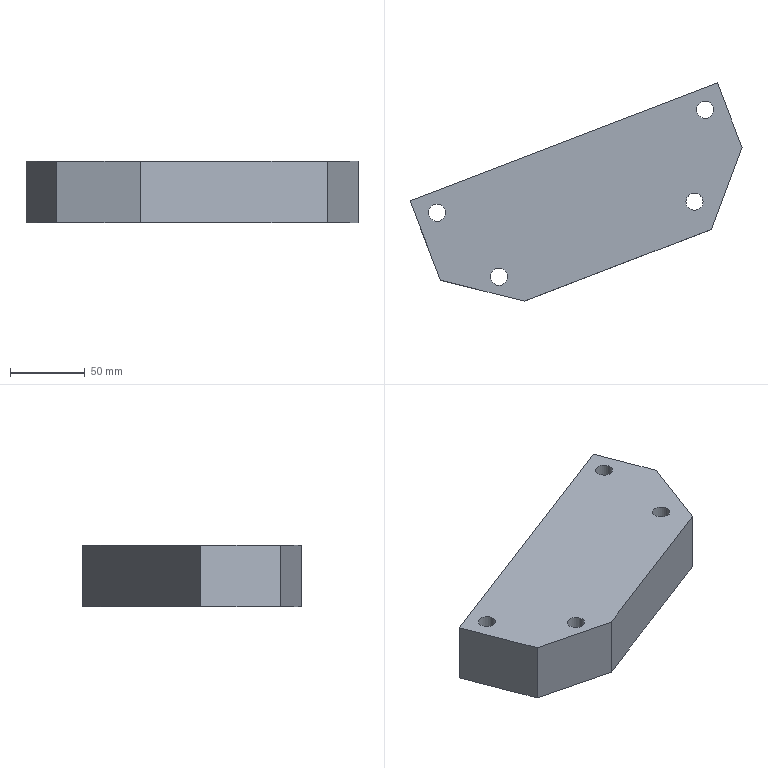Part | NX | features solid 2 | 1 solid | 20 faces | box 221.896 x 145.899 x 41 mm | volume 719760 mm3 | plane 12 | cylinder 8 | commonest cylinder face diameters 11.5 x4 18 x4
STEP:
#1=CARTESIAN_POINT('',(970.121,174.216,73.));
#2=VERTEX_POINT('',#1);
#3=CARTESIAN_POINT('',(968.06,179.584,73.));
#4=DIRECTION('',(0.,0.,-1.));
#5=DIRECTION('',(0.3584,-0.9336,0.));
#6=AXIS2_PLACEMENT_3D('',#3,#4,#5);
#7=CIRCLE('',#6,5.75);
#8=EDGE_CURVE('',#2,#2,#7,.T.);
#9=ORIENTED_EDGE('',*,*,#8,.F.);
#10=EDGE_LOOP('',(#9));
#11=FACE_BOUND('',#10,.T.);
#12=CARTESIAN_POINT('',(971.285,171.182,73.));
#13=VERTEX_POINT('',#12);
#14=CARTESIAN_POINT('',(968.06,179.584,73.));
#15=DIRECTION('',(0.,0.,-1.));
#16=DIRECTION('',(0.3584,-0.9336,0.));
#17=AXIS2_PLACEMENT_3D('',#14,#15,#16);
#18=CIRCLE('',#17,9.);
#19=EDGE_CURVE('',#13,#13,#18,.T.);
#20=ORIENTED_EDGE('',*,*,#19,.T.);
#21=EDGE_LOOP('',(#20));
#22=FACE_BOUND('',#21,.T.);
#23=CARTESIAN_POINT('',(968.06,179.584,73.));
#24=DIRECTION('',(0.,0.,1.));
#25=DIRECTION('',(-0.3584,0.9336,0.));
#26=AXIS2_PLACEMENT_3D('',#23,#24,#25);
#27=PLANE('',#26);
#28=ADVANCED_FACE('',(#11,#22),#27,.F.);
#29=CARTESIAN_POINT('',(1011.473,131.478,73.));
#30=VERTEX_POINT('',#29);
#31=CARTESIAN_POINT('',(1009.413,136.846,73.));
#32=DIRECTION('',(0.,0.,-1.));
#33=DIRECTION('',(0.3584,-0.9336,0.));
#34=AXIS2_PLACEMENT_3D('',#31,#32,#33);
#35=CIRCLE('',#34,5.75);
#36=EDGE_CURVE('',#30,#30,#35,.T.);
#37=ORIENTED_EDGE('',*,*,#36,.F.);
#38=EDGE_LOOP('',(#37));
#39=FACE_BOUND('',#38,.T.);
#40=CARTESIAN_POINT('',(1012.638,128.444,73.));
#41=VERTEX_POINT('',#40);
#42=CARTESIAN_POINT('',(1009.413,136.846,73.));
#43=DIRECTION('',(0.,0.,-1.));
#44=DIRECTION('',(0.3584,-0.9336,0.));
#45=AXIS2_PLACEMENT_3D('',#42,#43,#44);
#46=CIRCLE('',#45,9.);
#47=EDGE_CURVE('',#41,#41,#46,.T.);
#48=ORIENTED_EDGE('',*,*,#47,.T.);
#49=EDGE_LOOP('',(#48));
#50=FACE_BOUND('',#49,.T.);
#51=CARTESIAN_POINT('',(1009.413,136.846,73.));
#52=DIRECTION('',(0.,0.,1.));
#53=DIRECTION('',(-0.3584,0.9336,0.));
#54=AXIS2_PLACEMENT_3D('',#51,#52,#53);
#55=PLANE('',#54);
#56=ADVANCED_FACE('',(#39,#50),#55,.F.);
#57=CARTESIAN_POINT('',(1149.368,243.023,73.));
#58=VERTEX_POINT('',#57);
#59=CARTESIAN_POINT('',(1147.307,248.391,73.));
#60=DIRECTION('',(0.,0.,-1.));
#61=DIRECTION('',(0.3584,-0.9336,0.));
#62=AXIS2_PLACEMENT_3D('',#59,#60,#61);
#63=CIRCLE('',#62,5.75);
#64=EDGE_CURVE('',#58,#58,#63,.T.);
#65=ORIENTED_EDGE('',*,*,#64,.F.);
#66=EDGE_LOOP('',(#65));
#67=FACE_BOUND('',#66,.T.);
#68=CARTESIAN_POINT('',(1150.533,239.989,73.));
#69=VERTEX_POINT('',#68);
#70=CARTESIAN_POINT('',(1147.307,248.391,73.));
#71=DIRECTION('',(0.,0.,-1.));
#72=DIRECTION('',(0.3584,-0.9336,0.));
#73=AXIS2_PLACEMENT_3D('',#70,#71,#72);
#74=CIRCLE('',#73,9.);
#75=EDGE_CURVE('',#69,#69,#74,.T.);
#76=ORIENTED_EDGE('',*,*,#75,.T.);
#77=EDGE_LOOP('',(#76));
#78=FACE_BOUND('',#77,.T.);
#79=CARTESIAN_POINT('',(1044.614,208.97,73.));
#80=DIRECTION('',(0.,0.,1.));
#81=DIRECTION('',(-0.3584,0.9336,0.));
#82=AXIS2_PLACEMENT_3D('',#79,#80,#81);
#83=PLANE('',#82);
#84=ADVANCED_FACE('',(#67,#78),#83,.F.);
#85=CARTESIAN_POINT('',(1026.418,120.579,60.));
#86=VERTEX_POINT('',#85);
#87=CARTESIAN_POINT('',(1026.418,120.579,101.));
#88=VERTEX_POINT('',#87);
#89=CARTESIAN_POINT('',(1026.418,120.579,-25.));
#90=DIRECTION('',(0.,0.,1.));
#91=VECTOR('',#90,1000.);
#92=LINE('',#89,#91);
#93=EDGE_CURVE('',#86,#88,#92,.T.);
#94=ORIENTED_EDGE('',*,*,#93,.T.);
#95=CARTESIAN_POINT('',(970.348,134.558,101.));
#96=VERTEX_POINT('',#95);
#97=CARTESIAN_POINT('',(1046.37,115.604,101.));
#98=DIRECTION('',(-0.9703,0.2419,0.));
#99=VECTOR('',#98,1000.);
#100=LINE('',#97,#99);
#101=EDGE_CURVE('',#88,#96,#100,.T.);
#102=ORIENTED_EDGE('',*,*,#101,.T.);
#103=CARTESIAN_POINT('',(970.348,134.558,60.));
#104=VERTEX_POINT('',#103);
#105=CARTESIAN_POINT('',(970.348,134.558,-25.));
#106=DIRECTION('',(0.,0.,-1.));
#107=VECTOR('',#106,1000.);
#108=LINE('',#105,#107);
#109=EDGE_CURVE('',#96,#104,#108,.T.);
#110=ORIENTED_EDGE('',*,*,#109,.T.);
#111=CARTESIAN_POINT('',(1046.37,115.604,60.));
#112=DIRECTION('',(0.9703,-0.2419,0.));
#113=VECTOR('',#112,1000.);
#114=LINE('',#111,#113);
#115=EDGE_CURVE('',#104,#86,#114,.T.);
#116=ORIENTED_EDGE('',*,*,#115,.T.);
#117=EDGE_LOOP('',(#94,#102,#110,#116));
#118=FACE_BOUND('',#117,.T.);
#119=CARTESIAN_POINT('',(1046.37,115.604,-25.));
#120=DIRECTION('',(0.2419,0.9703,0.));
#121=DIRECTION('',(0.,0.,1.));
#122=AXIS2_PLACEMENT_3D('',#119,#120,#121);
#123=PLANE('',#122);
#124=ADVANCED_FACE('',(#118),#123,.F.);
#125=CARTESIAN_POINT('',(949.973,187.637,101.));
#126=VERTEX_POINT('',#125);
#127=CARTESIAN_POINT('',(966.099,145.626,101.));
#128=DIRECTION('',(0.3584,-0.9336,0.));
#129=VECTOR('',#128,1000.);
#130=LINE('',#127,#129);
#131=EDGE_CURVE('',#126,#96,#130,.T.);
#132=ORIENTED_EDGE('',*,*,#131,.F.);
#133=CARTESIAN_POINT('',(949.973,187.637,60.));
#134=VERTEX_POINT('',#133);
#135=CARTESIAN_POINT('',(949.973,187.637,-25.));
#136=DIRECTION('',(0.,0.,1.));
#137=VECTOR('',#136,1000.);
#138=LINE('',#135,#137);
#139=EDGE_CURVE('',#134,#126,#138,.T.);
#140=ORIENTED_EDGE('',*,*,#139,.F.);
#141=CARTESIAN_POINT('',(966.099,145.626,60.));
#142=DIRECTION('',(-0.3584,0.9336,0.));
#143=VECTOR('',#142,1000.);
#144=LINE('',#141,#143);
#145=EDGE_CURVE('',#104,#134,#144,.T.);
#146=ORIENTED_EDGE('',*,*,#145,.F.);
#147=ORIENTED_EDGE('',*,*,#109,.F.);
#148=EDGE_LOOP('',(#132,#140,#146,#147));
#149=FACE_BOUND('',#148,.T.);
#150=CARTESIAN_POINT('',(966.099,145.626,-25.));
#151=DIRECTION('',(-0.9336,-0.3584,0.));
#152=DIRECTION('',(0.,0.,-1.));
#153=AXIS2_PLACEMENT_3D('',#150,#151,#152);
#154=PLANE('',#153);
#155=ADVANCED_FACE('',(#149),#154,.T.);
#156=CARTESIAN_POINT('',(1155.36,266.478,60.));
#157=VERTEX_POINT('',#156);
#158=CARTESIAN_POINT('',(1155.36,266.478,101.));
#159=VERTEX_POINT('',#158);
#160=CARTESIAN_POINT('',(1155.36,266.478,-25.));
#161=DIRECTION('',(0.,0.,1.));
#162=VECTOR('',#161,1000.);
#163=LINE('',#160,#162);
#164=EDGE_CURVE('',#157,#159,#163,.T.);
#165=ORIENTED_EDGE('',*,*,#164,.F.);
#166=CARTESIAN_POINT('',(1001.32,207.347,60.));
#167=DIRECTION('',(0.9336,0.3584,0.));
#168=VECTOR('',#167,1000.);
#169=LINE('',#166,#168);
#170=EDGE_CURVE('',#134,#157,#169,.T.);
#171=ORIENTED_EDGE('',*,*,#170,.F.);
#172=ORIENTED_EDGE('',*,*,#139,.T.);
#173=CARTESIAN_POINT('',(1001.32,207.347,101.));
#174=DIRECTION('',(-0.9336,-0.3584,0.));
#175=VECTOR('',#174,1000.);
#176=LINE('',#173,#175);
#177=EDGE_CURVE('',#159,#126,#176,.T.);
#178=ORIENTED_EDGE('',*,*,#177,.F.);
#179=EDGE_LOOP('',(#165,#171,#172,#178));
#180=FACE_BOUND('',#179,.T.);
#181=CARTESIAN_POINT('',(1001.32,207.347,-25.));
#182=DIRECTION('',(-0.3584,0.9336,0.));
#183=DIRECTION('',(0.,0.,-1.));
#184=AXIS2_PLACEMENT_3D('',#181,#182,#183);
#185=PLANE('',#184);
#186=ADVANCED_FACE('',(#180),#185,.T.);
#187=CARTESIAN_POINT('',(1171.868,223.474,101.));
#188=VERTEX_POINT('',#187);
#189=CARTESIAN_POINT('',(1171.487,224.467,101.));
#190=DIRECTION('',(-0.3584,0.9336,0.));
#191=VECTOR('',#190,1000.);
#192=LINE('',#189,#191);
#193=EDGE_CURVE('',#188,#159,#192,.T.);
#194=ORIENTED_EDGE('',*,*,#193,.F.);
#195=CARTESIAN_POINT('',(1171.868,223.474,60.));
#196=VERTEX_POINT('',#195);
#197=CARTESIAN_POINT('',(1171.868,223.474,-25.));
#198=DIRECTION('',(0.,0.,-1.));
#199=VECTOR('',#198,1000.);
#200=LINE('',#197,#199);
#201=EDGE_CURVE('',#188,#196,#200,.T.);
#202=ORIENTED_EDGE('',*,*,#201,.T.);
#203=CARTESIAN_POINT('',(1171.487,224.467,60.));
#204=DIRECTION('',(0.3584,-0.9336,0.));
#205=VECTOR('',#204,1000.);
#206=LINE('',#203,#205);
#207=EDGE_CURVE('',#157,#196,#206,.T.);
#208=ORIENTED_EDGE('',*,*,#207,.F.);
#209=ORIENTED_EDGE('',*,*,#164,.T.);
#210=EDGE_LOOP('',(#194,#202,#208,#209));
#211=FACE_BOUND('',#210,.T.);
#212=CARTESIAN_POINT('',(1171.487,224.467,-25.));
#213=DIRECTION('',(0.9336,0.3584,0.));
#214=DIRECTION('',(0.,0.,1.));
#215=AXIS2_PLACEMENT_3D('',#212,#213,#214);
#216=PLANE('',#215);
#217=ADVANCED_FACE('',(#211),#216,.T.);
#218=CARTESIAN_POINT('',(1151.325,168.526,60.));
#219=VERTEX_POINT('',#218);
#220=CARTESIAN_POINT('',(1151.325,168.526,101.));
#221=VERTEX_POINT('',#220);
#222=CARTESIAN_POINT('',(1151.325,168.526,-25.));
#223=DIRECTION('',(0.,0.,1.));
#224=VECTOR('',#223,1000.);
#225=LINE('',#222,#224);
#226=EDGE_CURVE('',#219,#221,#225,.T.);
#227=ORIENTED_EDGE('',*,*,#226,.F.);
#228=CARTESIAN_POINT('',(746.976,-912.968,60.));
#229=DIRECTION('',(-0.3502,-0.9367,0.));
#230=VECTOR('',#229,1000.);
#231=LINE('',#228,#230);
#232=EDGE_CURVE('',#196,#219,#231,.T.);
#233=ORIENTED_EDGE('',*,*,#232,.F.);
#234=ORIENTED_EDGE('',*,*,#201,.F.);
#235=CARTESIAN_POINT('',(1234.634,391.351,101.));
#236=DIRECTION('',(0.3502,0.9367,0.));
#237=VECTOR('',#236,1000.);
#238=LINE('',#235,#237);
#239=EDGE_CURVE('',#221,#188,#238,.T.);
#240=ORIENTED_EDGE('',*,*,#239,.F.);
#241=EDGE_LOOP('',(#227,#233,#234,#240));
#242=FACE_BOUND('',#241,.T.);
#243=CARTESIAN_POINT('',(1145.984,154.243,93.));
#244=DIRECTION('',(0.9367,-0.3502,0.));
#245=DIRECTION('',(-0.3502,-0.9367,0.));
#246=AXIS2_PLACEMENT_3D('',#243,#244,#245);
#247=PLANE('',#246);
#248=ADVANCED_FACE('',(#242),#247,.T.);
#249=CARTESIAN_POINT('',(1033.573,123.325,60.));
#250=DIRECTION('',(-0.9336,-0.3584,0.));
#251=VECTOR('',#250,1000.);
#252=LINE('',#249,#251);
#253=EDGE_CURVE('',#219,#86,#252,.T.);
#254=ORIENTED_EDGE('',*,*,#253,.F.);
#255=ORIENTED_EDGE('',*,*,#226,.T.);
#256=CARTESIAN_POINT('',(1033.573,123.325,101.));
#257=DIRECTION('',(0.9336,0.3584,0.));
#258=VECTOR('',#257,1000.);
#259=LINE('',#256,#258);
#260=EDGE_CURVE('',#88,#221,#259,.T.);
#261=ORIENTED_EDGE('',*,*,#260,.F.);
#262=ORIENTED_EDGE('',*,*,#93,.F.);
#263=EDGE_LOOP('',(#254,#255,#261,#262));
#264=FACE_BOUND('',#263,.T.);
#265=CARTESIAN_POINT('',(1033.573,123.325,-25.));
#266=DIRECTION('',(0.3584,-0.9336,0.));
#267=DIRECTION('',(0.,0.,1.));
#268=AXIS2_PLACEMENT_3D('',#265,#266,#267);
#269=PLANE('',#268);
#270=ADVANCED_FACE('',(#264),#269,.T.);
#271=CARTESIAN_POINT('',(970.121,174.216,101.));
#272=VERTEX_POINT('',#271);
#273=CARTESIAN_POINT('',(968.06,179.584,101.));
#274=DIRECTION('',(0.,0.,-1.));
#275=DIRECTION('',(0.3584,-0.9336,0.));
#276=AXIS2_PLACEMENT_3D('',#273,#274,#275);
#277=CIRCLE('',#276,5.75);
#278=EDGE_CURVE('',#272,#272,#277,.T.);
#279=ORIENTED_EDGE('',*,*,#278,.F.);
#280=EDGE_LOOP('',(#279));
#281=FACE_BOUND('',#280,.T.);
#282=ORIENTED_EDGE('',*,*,#8,.T.);
#283=EDGE_LOOP('',(#282));
#284=FACE_BOUND('',#283,.T.);
#285=CARTESIAN_POINT('',(968.06,179.584,55.));
#286=DIRECTION('',(0.,0.,1.));
#287=DIRECTION('',(-0.3584,0.9336,0.));
#288=AXIS2_PLACEMENT_3D('',#285,#286,#287);
#289=CYLINDRICAL_SURFACE('',#288,5.75);
#290=ADVANCED_FACE('',(#281,#284),#289,.F.);
#291=CARTESIAN_POINT('',(1011.473,131.478,101.));
#292=VERTEX_POINT('',#291);
#293=CARTESIAN_POINT('',(1009.413,136.846,101.));
#294=DIRECTION('',(0.,0.,-1.));
#295=DIRECTION('',(0.3584,-0.9336,0.));
#296=AXIS2_PLACEMENT_3D('',#293,#294,#295);
#297=CIRCLE('',#296,5.75);
#298=EDGE_CURVE('',#292,#292,#297,.T.);
#299=ORIENTED_EDGE('',*,*,#298,.F.);
#300=EDGE_LOOP('',(#299));
#301=FACE_BOUND('',#300,.T.);
#302=ORIENTED_EDGE('',*,*,#36,.T.);
#303=EDGE_LOOP('',(#302));
#304=FACE_BOUND('',#303,.T.);
#305=CARTESIAN_POINT('',(1009.413,136.846,55.));
#306=DIRECTION('',(0.,0.,1.));
#307=DIRECTION('',(-0.3584,0.9336,0.));
#308=AXIS2_PLACEMENT_3D('',#305,#306,#307);
#309=CYLINDRICAL_SURFACE('',#308,5.75);
#310=ADVANCED_FACE('',(#301,#304),#309,.F.);
#311=CARTESIAN_POINT('',(1149.368,243.023,101.));
#312=VERTEX_POINT('',#311);
#313=CARTESIAN_POINT('',(1147.307,248.391,101.));
#314=DIRECTION('',(0.,0.,-1.));
#315=DIRECTION('',(0.3584,-0.9336,0.));
#316=AXIS2_PLACEMENT_3D('',#313,#314,#315);
#317=CIRCLE('',#316,5.75);
#318=EDGE_CURVE('',#312,#312,#317,.T.);
#319=ORIENTED_EDGE('',*,*,#318,.F.);
#320=EDGE_LOOP('',(#319));
#321=FACE_BOUND('',#320,.T.);
#322=ORIENTED_EDGE('',*,*,#64,.T.);
#323=EDGE_LOOP('',(#322));
#324=FACE_BOUND('',#323,.T.);
#325=CARTESIAN_POINT('',(1147.307,248.391,55.));
#326=DIRECTION('',(0.,0.,1.));
#327=DIRECTION('',(-0.3584,0.9336,0.));
#328=AXIS2_PLACEMENT_3D('',#325,#326,#327);
#329=CYLINDRICAL_SURFACE('',#328,5.75);
#330=ADVANCED_FACE('',(#321,#324),#329,.F.);
#331=CARTESIAN_POINT('',(1145.864,187.018,101.));
#332=VERTEX_POINT('',#331);
#333=CARTESIAN_POINT('',(1140.114,187.018,101.));
#334=DIRECTION('',(0.,0.,1.));
#335=DIRECTION('',(1.,0.,0.));
#336=AXIS2_PLACEMENT_3D('',#333,#334,#335);
#337=CIRCLE('',#336,5.75);
#338=EDGE_CURVE('',#332,#332,#337,.T.);
#339=ORIENTED_EDGE('',*,*,#338,.F.);
#340=EDGE_LOOP('',(#339));
#341=FACE_BOUND('',#340,.T.);
#342=ORIENTED_EDGE('',*,*,#318,.T.);
#343=EDGE_LOOP('',(#342));
#344=FACE_BOUND('',#343,.T.);
#345=ORIENTED_EDGE('',*,*,#298,.T.);
#346=EDGE_LOOP('',(#345));
#347=FACE_BOUND('',#346,.T.);
#348=ORIENTED_EDGE('',*,*,#278,.T.);
#349=EDGE_LOOP('',(#348));
#350=FACE_BOUND('',#349,.T.);
#351=ORIENTED_EDGE('',*,*,#260,.T.);
#352=ORIENTED_EDGE('',*,*,#239,.T.);
#353=ORIENTED_EDGE('',*,*,#193,.T.);
#354=ORIENTED_EDGE('',*,*,#177,.T.);
#355=ORIENTED_EDGE('',*,*,#131,.T.);
#356=ORIENTED_EDGE('',*,*,#101,.F.);
#357=EDGE_LOOP('',(#351,#352,#353,#354,#355,#356));
#358=FACE_BOUND('',#357,.T.);
#359=CARTESIAN_POINT('',(231.927,766.243,101.));
#360=DIRECTION('',(0.,0.,1.));
#361=DIRECTION('',(-0.3584,0.9336,0.));
#362=AXIS2_PLACEMENT_3D('',#359,#360,#361);
#363=PLANE('',#362);
#364=ADVANCED_FACE('',(#341,#344,#347,#350,#358),#363,.T.);
#365=ORIENTED_EDGE('',*,*,#47,.F.);
#366=EDGE_LOOP('',(#365));
#367=FACE_BOUND('',#366,.T.);
#368=CARTESIAN_POINT('',(1012.638,128.444,60.));
#369=VERTEX_POINT('',#368);
#370=CARTESIAN_POINT('',(1009.413,136.846,60.));
#371=DIRECTION('',(0.,0.,-1.));
#372=DIRECTION('',(0.3584,-0.9336,0.));
#373=AXIS2_PLACEMENT_3D('',#370,#371,#372);
#374=CIRCLE('',#373,9.);
#375=EDGE_CURVE('',#369,#369,#374,.T.);
#376=ORIENTED_EDGE('',*,*,#375,.T.);
#377=EDGE_LOOP('',(#376));
#378=FACE_BOUND('',#377,.T.);
#379=CARTESIAN_POINT('',(1009.413,136.846,60.));
#380=DIRECTION('',(0.,0.,1.));
#381=DIRECTION('',(-0.3584,0.9336,0.));
#382=AXIS2_PLACEMENT_3D('',#379,#380,#381);
#383=CYLINDRICAL_SURFACE('',#382,9.);
#384=ADVANCED_FACE('',(#367,#378),#383,.F.);
#385=ORIENTED_EDGE('',*,*,#75,.F.);
#386=EDGE_LOOP('',(#385));
#387=FACE_BOUND('',#386,.T.);
#388=CARTESIAN_POINT('',(1150.533,239.989,60.));
#389=VERTEX_POINT('',#388);
#390=CARTESIAN_POINT('',(1147.307,248.391,60.));
#391=DIRECTION('',(0.,0.,-1.));
#392=DIRECTION('',(0.3584,-0.9336,0.));
#393=AXIS2_PLACEMENT_3D('',#390,#391,#392);
#394=CIRCLE('',#393,9.);
#395=EDGE_CURVE('',#389,#389,#394,.T.);
#396=ORIENTED_EDGE('',*,*,#395,.T.);
#397=EDGE_LOOP('',(#396));
#398=FACE_BOUND('',#397,.T.);
#399=CARTESIAN_POINT('',(1147.307,248.391,60.));
#400=DIRECTION('',(0.,0.,1.));
#401=DIRECTION('',(-0.3584,0.9336,0.));
#402=AXIS2_PLACEMENT_3D('',#399,#400,#401);
#403=CYLINDRICAL_SURFACE('',#402,9.);
#404=ADVANCED_FACE('',(#387,#398),#403,.F.);
#405=ORIENTED_EDGE('',*,*,#19,.F.);
#406=EDGE_LOOP('',(#405));
#407=FACE_BOUND('',#406,.T.);
#408=CARTESIAN_POINT('',(971.285,171.182,60.));
#409=VERTEX_POINT('',#408);
#410=CARTESIAN_POINT('',(968.06,179.584,60.));
#411=DIRECTION('',(0.,0.,-1.));
#412=DIRECTION('',(0.3584,-0.9336,0.));
#413=AXIS2_PLACEMENT_3D('',#410,#411,#412);
#414=CIRCLE('',#413,9.);
#415=EDGE_CURVE('',#409,#409,#414,.T.);
#416=ORIENTED_EDGE('',*,*,#415,.T.);
#417=EDGE_LOOP('',(#416));
#418=FACE_BOUND('',#417,.T.);
#419=CARTESIAN_POINT('',(968.06,179.584,60.));
#420=DIRECTION('',(0.,0.,1.));
#421=DIRECTION('',(-0.3584,0.9336,0.));
#422=AXIS2_PLACEMENT_3D('',#419,#420,#421);
#423=CYLINDRICAL_SURFACE('',#422,9.);
#424=ADVANCED_FACE('',(#407,#418),#423,.F.);
#425=CARTESIAN_POINT('',(1149.114,187.018,60.));
#426=VERTEX_POINT('',#425);
#427=CARTESIAN_POINT('',(1140.114,187.018,60.));
#428=DIRECTION('',(0.,0.,-1.));
#429=DIRECTION('',(1.,0.,0.));
#430=AXIS2_PLACEMENT_3D('',#427,#428,#429);
#431=CIRCLE('',#430,9.);
#432=EDGE_CURVE('',#426,#426,#431,.T.);
#433=ORIENTED_EDGE('',*,*,#432,.F.);
#434=EDGE_LOOP('',(#433));
#435=FACE_BOUND('',#434,.T.);
#436=ORIENTED_EDGE('',*,*,#415,.F.);
#437=EDGE_LOOP('',(#436));
#438=FACE_BOUND('',#437,.T.);
#439=ORIENTED_EDGE('',*,*,#395,.F.);
#440=EDGE_LOOP('',(#439));
#441=FACE_BOUND('',#440,.T.);
#442=ORIENTED_EDGE('',*,*,#375,.F.);
#443=EDGE_LOOP('',(#442));
#444=FACE_BOUND('',#443,.T.);
#445=ORIENTED_EDGE('',*,*,#207,.T.);
#446=ORIENTED_EDGE('',*,*,#232,.T.);
#447=ORIENTED_EDGE('',*,*,#253,.T.);
#448=ORIENTED_EDGE('',*,*,#115,.F.);
#449=ORIENTED_EDGE('',*,*,#145,.T.);
#450=ORIENTED_EDGE('',*,*,#170,.T.);
#451=EDGE_LOOP('',(#445,#446,#447,#448,#449,#450));
#452=FACE_BOUND('',#451,.T.);
#453=CARTESIAN_POINT('',(1139.595,-1059.76,60.));
#454=DIRECTION('',(0.,0.,1.));
#455=DIRECTION('',(-0.3584,0.9336,0.));
#456=AXIS2_PLACEMENT_3D('',#453,#454,#455);
#457=PLANE('',#456);
#458=ADVANCED_FACE('',(#435,#438,#441,#444,#452),#457,.F.);
#459=CARTESIAN_POINT('',(1142.175,181.65,73.));
#460=VERTEX_POINT('',#459);
#461=CARTESIAN_POINT('',(1140.114,187.018,73.));
#462=DIRECTION('',(0.,0.,-1.));
#463=DIRECTION('',(0.3584,-0.9336,0.));
#464=AXIS2_PLACEMENT_3D('',#461,#462,#463);
#465=CIRCLE('',#464,5.75);
#466=EDGE_CURVE('',#460,#460,#465,.T.);
#467=ORIENTED_EDGE('',*,*,#466,.F.);
#468=EDGE_LOOP('',(#467));
#469=FACE_BOUND('',#468,.T.);
#470=CARTESIAN_POINT('',(1143.339,178.615,73.));
#471=VERTEX_POINT('',#470);
#472=CARTESIAN_POINT('',(1140.114,187.018,73.));
#473=DIRECTION('',(0.,0.,-1.));
#474=DIRECTION('',(0.3584,-0.9336,0.));
#475=AXIS2_PLACEMENT_3D('',#472,#473,#474);
#476=CIRCLE('',#475,9.);
#477=EDGE_CURVE('',#471,#471,#476,.T.);
#478=ORIENTED_EDGE('',*,*,#477,.T.);
#479=EDGE_LOOP('',(#478));
#480=FACE_BOUND('',#479,.T.);
#481=CARTESIAN_POINT('',(1140.114,187.018,73.));
#482=DIRECTION('',(0.,0.,1.));
#483=DIRECTION('',(-0.3584,0.9336,0.));
#484=AXIS2_PLACEMENT_3D('',#481,#482,#483);
#485=PLANE('',#484);
#486=ADVANCED_FACE('',(#469,#480),#485,.F.);
#487=ORIENTED_EDGE('',*,*,#338,.T.);
#488=EDGE_LOOP('',(#487));
#489=FACE_BOUND('',#488,.T.);
#490=ORIENTED_EDGE('',*,*,#466,.T.);
#491=EDGE_LOOP('',(#490));
#492=FACE_BOUND('',#491,.T.);
#493=CARTESIAN_POINT('',(1140.114,187.018,55.));
#494=DIRECTION('',(0.,0.,1.));
#495=DIRECTION('',(-0.3584,0.9336,0.));
#496=AXIS2_PLACEMENT_3D('',#493,#494,#495);
#497=CYLINDRICAL_SURFACE('',#496,5.75);
#498=ADVANCED_FACE('',(#489,#492),#497,.F.);
#499=ORIENTED_EDGE('',*,*,#477,.F.);
#500=EDGE_LOOP('',(#499));
#501=FACE_BOUND('',#500,.T.);
#502=ORIENTED_EDGE('',*,*,#432,.T.);
#503=EDGE_LOOP('',(#502));
#504=FACE_BOUND('',#503,.T.);
#505=CARTESIAN_POINT('',(1140.114,187.018,60.));
#506=DIRECTION('',(0.,0.,1.));
#507=DIRECTION('',(-0.3584,0.9336,0.));
#508=AXIS2_PLACEMENT_3D('',#505,#506,#507);
#509=CYLINDRICAL_SURFACE('',#508,9.);
#510=ADVANCED_FACE('',(#501,#504),#509,.F.);
#511=CLOSED_SHELL('',(#28,#56,#84,#124,#155,#186,#217,#248,#270,#290,#310,#330,#364,#384,#404,#424,#458,#486,#498,#510));
#512=MANIFOLD_SOLID_BREP('',#511);
#513=(LENGTH_UNIT()NAMED_UNIT(*)SI_UNIT(.MILLI.,.METRE.));
#514=UNCERTAINTY_MEASURE_WITH_UNIT(LENGTH_MEASURE(0.00001),#513,'','');
#515=(NAMED_UNIT(*)PLANE_ANGLE_UNIT()SI_UNIT($,.RADIAN.));
#516=(NAMED_UNIT(*)SI_UNIT($,.STERADIAN.)SOLID_ANGLE_UNIT());
#517=(GEOMETRIC_REPRESENTATION_CONTEXT(3)GLOBAL_UNCERTAINTY_ASSIGNED_CONTEXT((#514))GLOBAL_UNIT_ASSIGNED_CONTEXT((#513,#515,#516))REPRESENTATION_CONTEXT('',''));
#518=ADVANCED_BREP_SHAPE_REPRESENTATION('',(#512),#517);